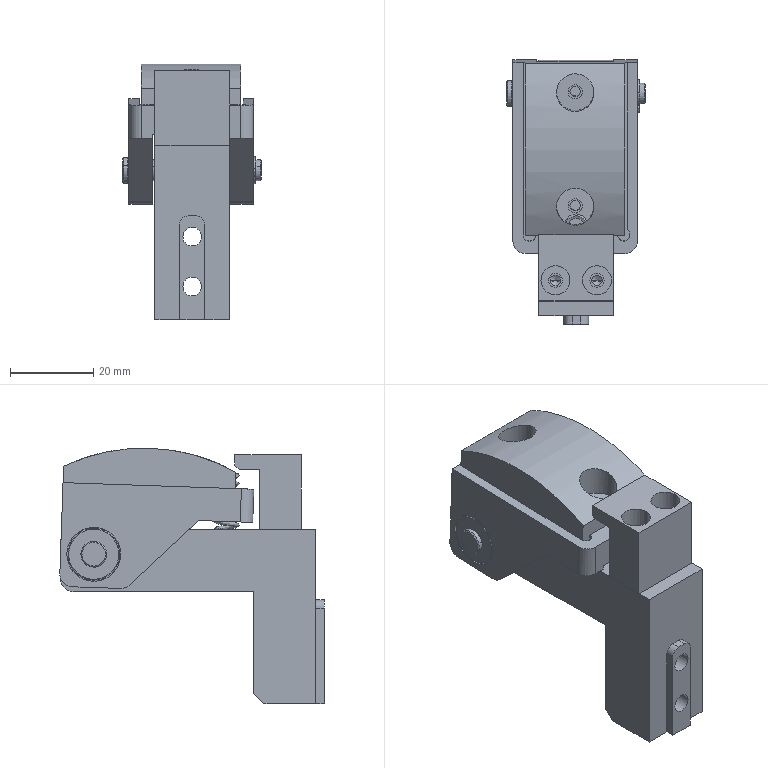Part | NX | features BREP 9 | 9 solids | 224 faces | box 33.4 x 63.67 x 61.571 mm | volume 45572 mm3 | cylinder 106 | plane 74 | cone 22 | torus 20 | spline 2 | commonest cylinder face diameters 5 x12 2.5 x10 3.4 x8 6 x8 11 x8 7 x6